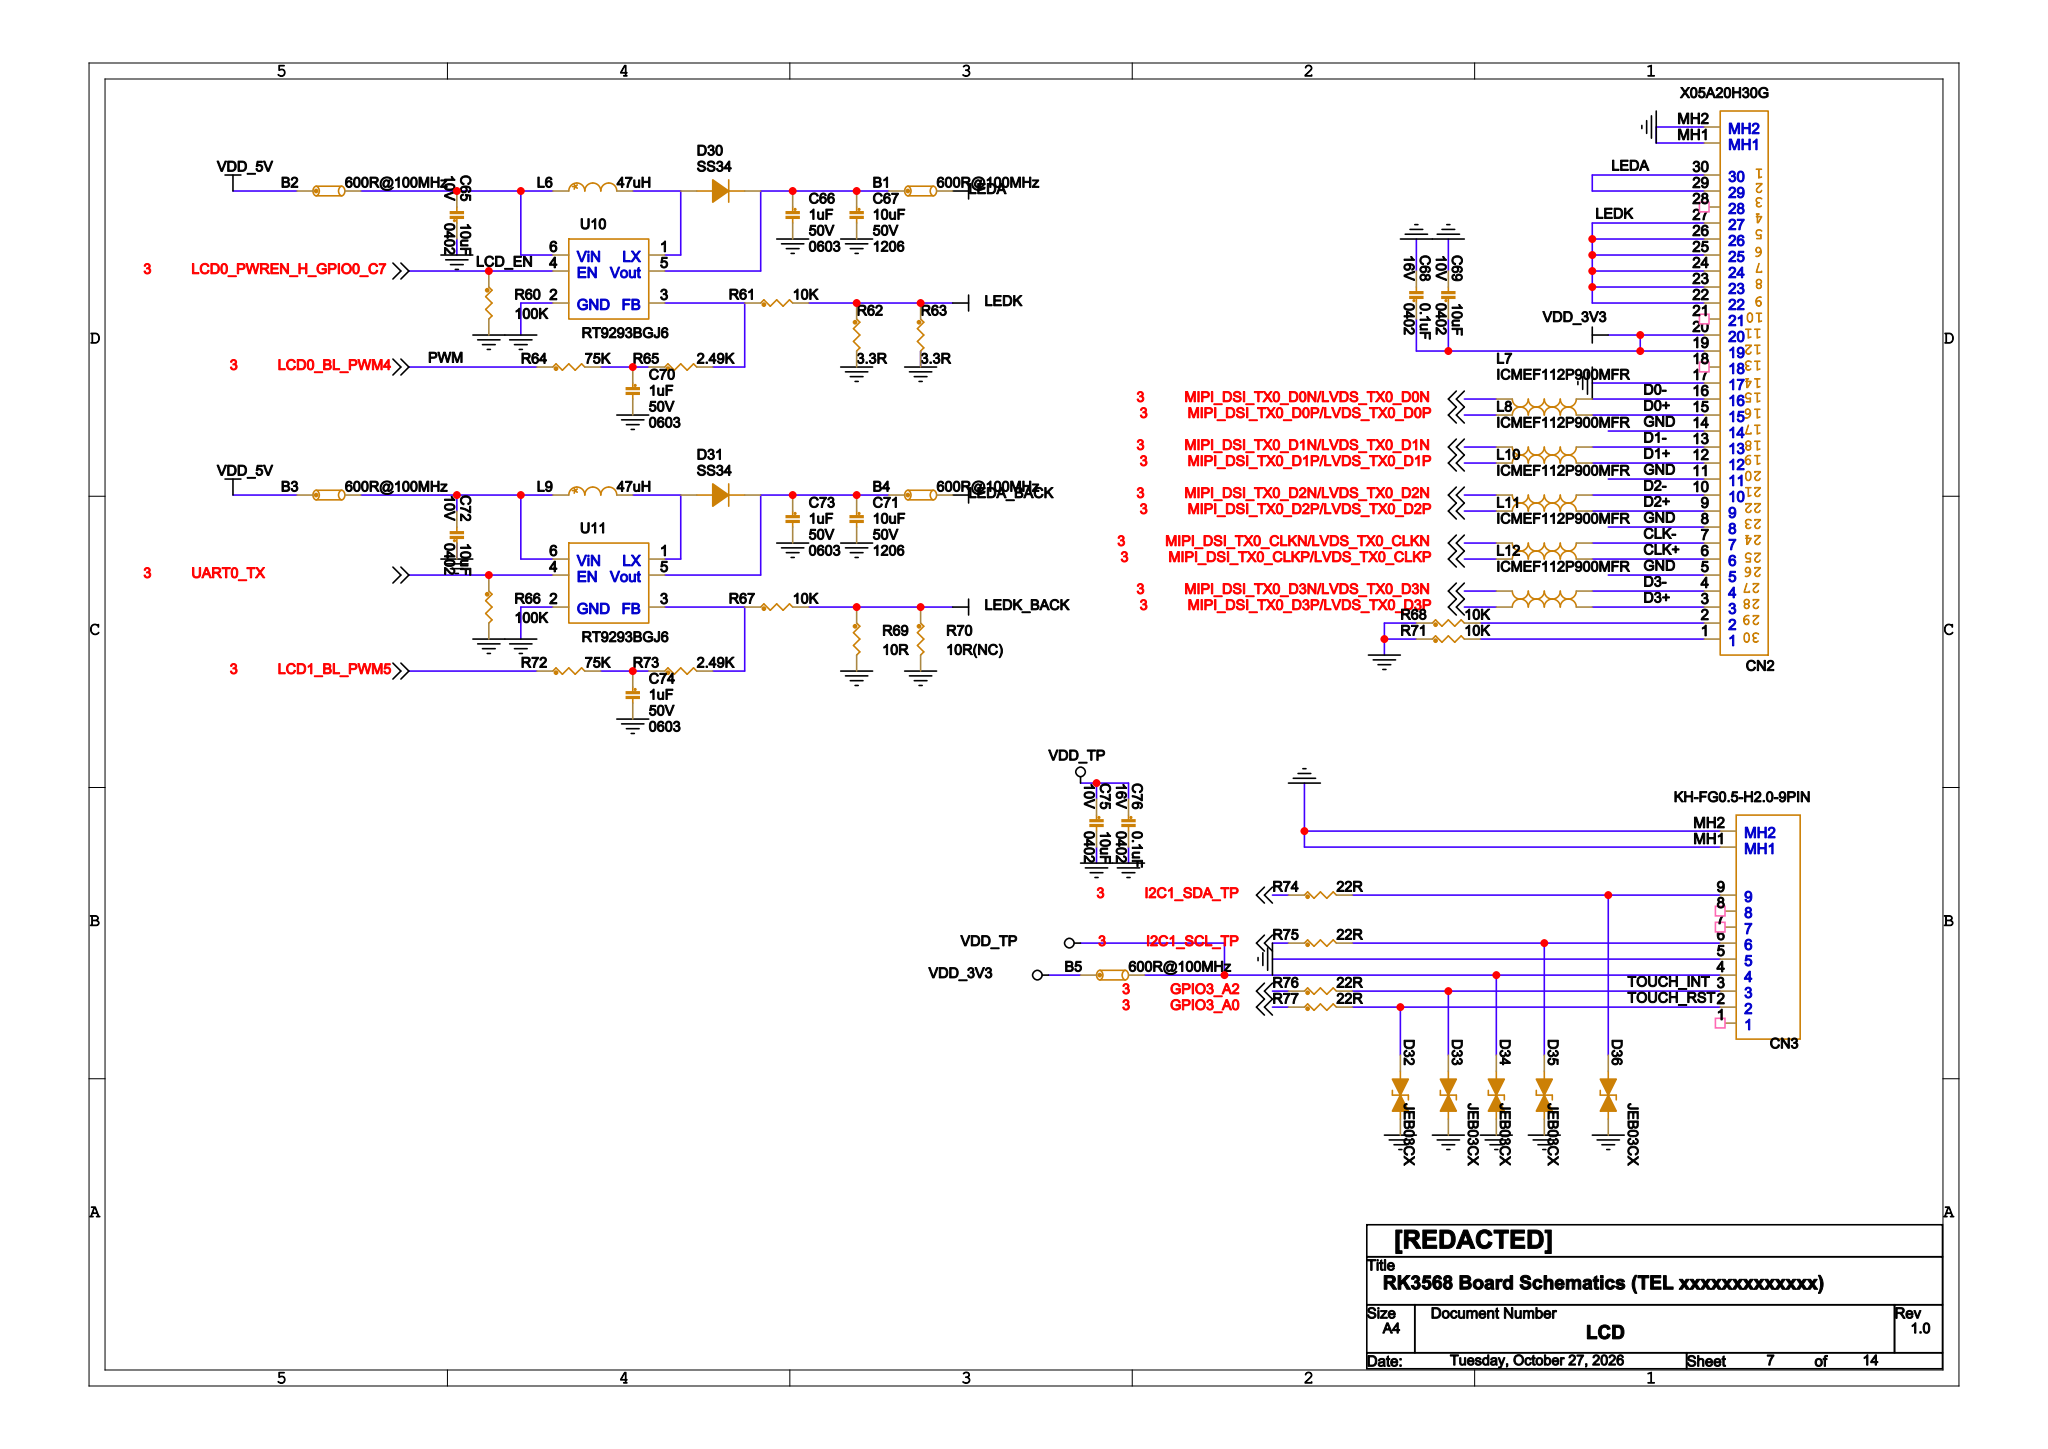Circuit board | Cadence Allegro | 669 parts | 581 nets | one sheet of the schematic
Parts on this sheet (reference | value | footprint):
B1 | 600R@100MHz | R0805
B2 | 600R@100MHz | R0805
B3 | 600R@100MHz | R0805
B4 | 600R@100MHz | R0805
B5 | 600R@100MHz | R0805
C65 | 10uF | C0402
C66 | 1uF | C0603
C67 | 10uF | C1206
C68 | 0.1uF | C0402
C69 | 10uF | C0402
C70 | 1uF | C0603
C71 | 10uF | C1206
C72 | 10uF | C0402
C73 | 1uF | C0603
C74 | 1uF | C0603
C75 | 10uF | C0402
C76 | 0.1uF | C0402
CN2 | X05A20H30G | FPC-30-0P5-2MMH
CN3 | KH-FG0.5-H2.0-9PIN | FPC-9-0P5-2MMH
D30 | SS34 | SMA
D31 | SS34 | SMA
D32 | JEB03CX | SOD323
D33 | JEB03CX | SOD323
D34 | JEB03CX | SOD323
D35 | JEB03CX | SOD323
D36 | JEB03CX | SOD323
L6 | 47uH | IND5X5
L7 | ICMEF112P900MFR | ICMEF112P900MFR
L8 | ICMEF112P900MFR | ICMEF112P900MFR
L9 | 47uH | IND5X5
L10 | ICMEF112P900MFR | ICMEF112P900MFR
L11 | ICMEF112P900MFR | ICMEF112P900MFR
L12 | ICMEF112P900MFR | ICMEF112P900MFR
R60 | 100K | R0402
R61 | 10K | R0402
R62 | 3.3R | R0603
R63 | 3.3R | R0603
R64 | 75K | R0402
R65 | 2.49K | R0402
R66 | 100K | R0402
R67 | 10K | R0402
R68 | 10K | R0402
R69 | 10R | R0603
R70 | 10R(NC) | R0603
R71 | 10K | R0402
R72 | 75K | R0402
R73 | 2.49K | R0402
R74 | 22R | R0402
R75 | 22R | R0402
R76 | 22R | R0402
R77 | 22R | R0402
U10 | RT9293BGJ6 | SOT23-6
U11 | RT9293BGJ6 | SOT23-6
Nets of these parts (net: part-pin ...):
GND: C65-1 C66-2 C67-2 C68-2 C69-2 C70-2 C71-2 C72-1 C73-2 C74-2 C75-2 C76-2 CN3-5 CN3-MH1 CN3-MH2 D32-1 D33-1 D34-1 D35-1 D36-1 L7-5 L7-6 L8-5 L8-6 L10-5 L10-6 L11-5 L11-6 L12-5 L12-6 R60-2 R62-2 R63-2 R66-2 R68-1 R69-2 R70-2 R71-1 U10-2 U11-2 CN2-5 CN2-8 CN2-11 CN2-14 CN2-17 CN2-MH1 CN2-MH2
VDD_5V: B2-1 B3-1
VCC3V3_SYS: B5-1 C68-1 C69-1 CN2-19 CN2-20
N84564969: B1-1 C66-1 C67-1 D30-2 U10-5
LEDA: B1-2 CN2-29 CN2-30
N84564879: B2-2 C65-2 L6-1 U10-6
N84582394: B3-2 C72-2 L9-1 U11-6
N84582456: B4-1 C71-1 C73-1 D31-2 U11-5
LEDA_BACK: B4-2
VDD_TP: B5-2 C75-1 C76-1 CN3-4 D34-2
N84565027: C70-1 R64-2 R65-1
N84582526: C74-1 R72-2 R73-1
N84199090: R71-2 CN2-1
D2-: L10-1 CN2-10
D1+: L8-2 CN2-12
D1-: L8-1 CN2-13
D0+: L7-2 CN2-15
D0-: L7-1 CN2-16
N84199088: R68-2 CN2-2
LEDK: R61-2 R62-1 R63-1 CN2-22 CN2-23 CN2-24 CN2-25 CN2-26 CN2-27
D3+: L12-2 CN2-3
D3-: L12-1 CN2-4
CLK+: L11-2 CN2-6
CLK-: L11-1 CN2-7
D2+: L10-2 CN2-9
TOUCH_RST: CN3-2 D32-2 R77-2
TOUCH_INT: CN3-3 D33-2 R76-2
N84322351: CN3-6 D35-2 R75-2
N84322344: CN3-9 D36-2 R74-2
LEDK_BACK: R67-2 R69-1 R70-1
N84564901: D30-1 L6-2 U10-1
N84582414: D31-1 L9-2 U11-1
MIPI_DSI_TX0_D2N/LVDS_TX0_D2N: L10-3
MIPI_DSI_TX0_D2P/LVDS_TX0_D2P: L10-4
MIPI_DSI_TX0_CLKN/LVDS_TX0_CLKN: L11-3
MIPI_DSI_TX0_CLKP/LVDS_TX0_CLKP: L11-4
MIPI_DSI_TX0_D3N/LVDS_TX0_D3N: L12-3
MIPI_DSI_TX0_D3P/LVDS_TX0_D3P: L12-4
MIPI_DSI_TX0_D0N/LVDS_TX0_D0N: L7-3
MIPI_DSI_TX0_D0P/LVDS_TX0_D0P: L7-4
MIPI_DSI_TX0_D1N/LVDS_TX0_D1N: L8-3
MIPI_DSI_TX0_D1P/LVDS_TX0_D1P: L8-4
I2C1_SDA_TP: R74-1
I2C1_SCL_TP: R75-1
GPIO3_A2: R76-1
GPIO3_A0: R77-1
N84564907: R61-1 R65-2 U10-3
N84582418: R67-1 R73-2 U11-3
LCD0_PWREN_H_GPIO0_C7: R60-1 U10-4
UART0_TX: R66-1 U11-4
LCD0_BL_PWM4: R64-1
LCD1_BL_PWM5: R72-1